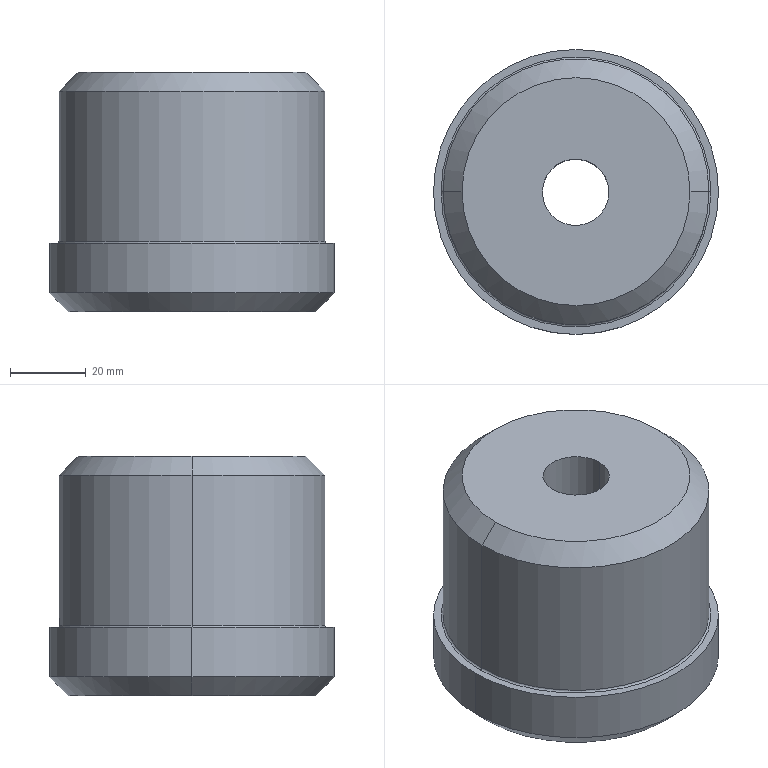Part | SolidWorks | features 3DProfileFeature 1, Chamfer 1, Extrusion 1, Fillet 1, HoleWzd 1, ICE 1 | 1 solid | 15 faces | box 75 x 75 x 63 mm | volume 232128 mm3 | cylinder 6 | cone 4 | plane 3 | torus 2 | commonest cylinder face diameters 17.5 x2 70 x2 75 x2
STEP:
#1=CARTESIAN_POINT('',(35.5,0.,0.));
#2=VERTEX_POINT('',#1);
#3=CARTESIAN_POINT('',(-35.5,0.,0.));
#4=VERTEX_POINT('',#3);
#5=CARTESIAN_POINT('',(0.,0.,0.));
#6=DIRECTION('',(0.,0.,-1.));
#7=DIRECTION('',(-1.,0.,0.));
#8=AXIS2_PLACEMENT_3D('',#5,#6,#7);
#9=CIRCLE('',#8,35.5);
#10=EDGE_CURVE('',#2,#4,#9,.T.);
#11=ORIENTED_EDGE('',*,*,#10,.F.);
#12=CARTESIAN_POINT('',(35.,0.,0.5));
#13=VERTEX_POINT('',#12);
#14=CARTESIAN_POINT('',(35.5,0.,0.5));
#15=DIRECTION('',(0.,1.,0.));
#16=DIRECTION('',(-1.,0.,0.));
#17=AXIS2_PLACEMENT_3D('',#14,#15,#16);
#18=CIRCLE('',#17,0.5);
#19=EDGE_CURVE('',#2,#13,#18,.T.);
#20=ORIENTED_EDGE('',*,*,#19,.T.);
#21=CARTESIAN_POINT('',(-35.,0.,0.5));
#22=VERTEX_POINT('',#21);
#23=CARTESIAN_POINT('',(0.,0.,0.5));
#24=DIRECTION('',(0.,0.,1.));
#25=DIRECTION('',(-1.,0.,0.));
#26=AXIS2_PLACEMENT_3D('',#23,#24,#25);
#27=CIRCLE('',#26,35.);
#28=EDGE_CURVE('',#22,#13,#27,.T.);
#29=ORIENTED_EDGE('',*,*,#28,.F.);
#30=CARTESIAN_POINT('',(-35.5,0.,0.5));
#31=DIRECTION('',(0.,-1.,0.));
#32=DIRECTION('',(0.,0.,-1.));
#33=AXIS2_PLACEMENT_3D('',#30,#31,#32);
#34=CIRCLE('',#33,0.5);
#35=EDGE_CURVE('',#4,#22,#34,.T.);
#36=ORIENTED_EDGE('',*,*,#35,.F.);
#37=EDGE_LOOP('',(#11,#20,#29,#36));
#38=FACE_OUTER_BOUND('',#37,.T.);
#39=CARTESIAN_POINT('',(0.,0.,0.5));
#40=DIRECTION('',(0.,0.,-1.));
#41=DIRECTION('',(-1.,0.,0.));
#42=AXIS2_PLACEMENT_3D('',#39,#40,#41);
#43=TOROIDAL_SURFACE('',#42,35.5,0.5);
#44=ADVANCED_FACE('',(#38),#43,.F.);
#45=CARTESIAN_POINT('',(-8.843,-0.1401,-18.));
#46=VERTEX_POINT('',#45);
#47=CARTESIAN_POINT('',(8.657,-0.1401,-18.));
#48=VERTEX_POINT('',#47);
#49=CARTESIAN_POINT('',(-0.09343,-0.1401,-18.));
#50=DIRECTION('',(0.,0.,1.));
#51=DIRECTION('',(1.,0.,0.));
#52=AXIS2_PLACEMENT_3D('',#49,#50,#51);
#53=CIRCLE('',#52,8.75);
#54=EDGE_CURVE('',#46,#48,#53,.T.);
#55=ORIENTED_EDGE('',*,*,#54,.F.);
#56=CARTESIAN_POINT('',(-8.843,-0.1401,45.));
#57=VERTEX_POINT('',#56);
#58=CARTESIAN_POINT('',(-8.843,-0.1401,45.));
#59=DIRECTION('',(0.,0.,1.));
#60=VECTOR('',#59,1000.);
#61=LINE('',#58,#60);
#62=EDGE_CURVE('',#46,#57,#61,.T.);
#63=ORIENTED_EDGE('',*,*,#62,.T.);
#64=CARTESIAN_POINT('',(8.657,-0.1401,45.));
#65=VERTEX_POINT('',#64);
#66=CARTESIAN_POINT('',(-0.09343,-0.1401,45.));
#67=DIRECTION('',(0.,0.,1.));
#68=DIRECTION('',(1.,0.,0.));
#69=AXIS2_PLACEMENT_3D('',#66,#67,#68);
#70=CIRCLE('',#69,8.75);
#71=EDGE_CURVE('',#57,#65,#70,.T.);
#72=ORIENTED_EDGE('',*,*,#71,.T.);
#73=CARTESIAN_POINT('',(8.657,-0.1401,45.));
#74=DIRECTION('',(0.,0.,1.));
#75=VECTOR('',#74,1000.);
#76=LINE('',#73,#75);
#77=EDGE_CURVE('',#48,#65,#76,.T.);
#78=ORIENTED_EDGE('',*,*,#77,.F.);
#79=EDGE_LOOP('',(#55,#63,#72,#78));
#80=FACE_OUTER_BOUND('',#79,.T.);
#81=CARTESIAN_POINT('',(-0.09343,-0.1401,45.));
#82=DIRECTION('',(0.,0.,1.));
#83=DIRECTION('',(1.,0.,0.));
#84=AXIS2_PLACEMENT_3D('',#81,#82,#83);
#85=CYLINDRICAL_SURFACE('',#84,8.75);
#86=ADVANCED_FACE('',(#80),#85,.F.);
#87=CARTESIAN_POINT('',(-32.5,0.,-18.));
#88=VERTEX_POINT('',#87);
#89=CARTESIAN_POINT('',(32.5,0.,-18.));
#90=VERTEX_POINT('',#89);
#91=CARTESIAN_POINT('',(0.,0.,-18.));
#92=DIRECTION('',(0.,0.,-1.));
#93=DIRECTION('',(-1.,0.,0.));
#94=AXIS2_PLACEMENT_3D('',#91,#92,#93);
#95=CIRCLE('',#94,32.5);
#96=EDGE_CURVE('',#88,#90,#95,.T.);
#97=ORIENTED_EDGE('',*,*,#96,.F.);
#98=CARTESIAN_POINT('',(-37.5,0.,-13.));
#99=VERTEX_POINT('',#98);
#100=CARTESIAN_POINT('',(-32.5,0.,-18.));
#101=DIRECTION('',(-0.7071,0.,0.7071));
#102=VECTOR('',#101,1000.);
#103=LINE('',#100,#102);
#104=EDGE_CURVE('',#88,#99,#103,.T.);
#105=ORIENTED_EDGE('',*,*,#104,.T.);
#106=CARTESIAN_POINT('',(37.5,0.,-13.));
#107=VERTEX_POINT('',#106);
#108=CARTESIAN_POINT('',(0.,0.,-13.));
#109=DIRECTION('',(0.,0.,1.));
#110=DIRECTION('',(-1.,0.,0.));
#111=AXIS2_PLACEMENT_3D('',#108,#109,#110);
#112=CIRCLE('',#111,37.5);
#113=EDGE_CURVE('',#107,#99,#112,.T.);
#114=ORIENTED_EDGE('',*,*,#113,.F.);
#115=CARTESIAN_POINT('',(32.5,0.,-18.));
#116=DIRECTION('',(0.7071,0.,0.7071));
#117=VECTOR('',#116,1000.);
#118=LINE('',#115,#117);
#119=EDGE_CURVE('',#90,#107,#118,.T.);
#120=ORIENTED_EDGE('',*,*,#119,.F.);
#121=EDGE_LOOP('',(#97,#105,#114,#120));
#122=FACE_OUTER_BOUND('',#121,.T.);
#123=CARTESIAN_POINT('',(0.,0.,-18.));
#124=DIRECTION('',(0.,0.,1.));
#125=DIRECTION('',(1.,0.,0.));
#126=AXIS2_PLACEMENT_3D('',#123,#124,#125);
#127=CONICAL_SURFACE('',#126,32.5,0.7854);
#128=ADVANCED_FACE('',(#122),#127,.T.);
#129=CARTESIAN_POINT('',(30.,0.,45.));
#130=VERTEX_POINT('',#129);
#131=CARTESIAN_POINT('',(-30.,0.,45.));
#132=VERTEX_POINT('',#131);
#133=CARTESIAN_POINT('',(0.,0.,45.));
#134=DIRECTION('',(0.,0.,1.));
#135=DIRECTION('',(1.,0.,0.));
#136=AXIS2_PLACEMENT_3D('',#133,#134,#135);
#137=CIRCLE('',#136,30.);
#138=EDGE_CURVE('',#130,#132,#137,.T.);
#139=ORIENTED_EDGE('',*,*,#138,.F.);
#140=CARTESIAN_POINT('',(35.,0.,40.));
#141=VERTEX_POINT('',#140);
#142=CARTESIAN_POINT('',(30.,0.,45.));
#143=DIRECTION('',(0.7071,0.,-0.7071));
#144=VECTOR('',#143,1000.);
#145=LINE('',#142,#144);
#146=EDGE_CURVE('',#130,#141,#145,.T.);
#147=ORIENTED_EDGE('',*,*,#146,.T.);
#148=CARTESIAN_POINT('',(-35.,0.,40.));
#149=VERTEX_POINT('',#148);
#150=CARTESIAN_POINT('',(0.,0.,40.));
#151=DIRECTION('',(0.,0.,-1.));
#152=DIRECTION('',(1.,0.,0.));
#153=AXIS2_PLACEMENT_3D('',#150,#151,#152);
#154=CIRCLE('',#153,35.);
#155=EDGE_CURVE('',#149,#141,#154,.T.);
#156=ORIENTED_EDGE('',*,*,#155,.F.);
#157=CARTESIAN_POINT('',(-30.,0.,45.));
#158=DIRECTION('',(-0.7071,0.,-0.7071));
#159=VECTOR('',#158,1000.);
#160=LINE('',#157,#159);
#161=EDGE_CURVE('',#132,#149,#160,.T.);
#162=ORIENTED_EDGE('',*,*,#161,.F.);
#163=EDGE_LOOP('',(#139,#147,#156,#162));
#164=FACE_OUTER_BOUND('',#163,.T.);
#165=CARTESIAN_POINT('',(0.,0.,45.));
#166=DIRECTION('',(0.,0.,-1.));
#167=DIRECTION('',(-1.,0.,0.));
#168=AXIS2_PLACEMENT_3D('',#165,#166,#167);
#169=CONICAL_SURFACE('',#168,30.,0.7854);
#170=ADVANCED_FACE('',(#164),#169,.T.);
#171=ORIENTED_EDGE('',*,*,#113,.T.);
#172=CARTESIAN_POINT('',(-37.5,0.,0.));
#173=VERTEX_POINT('',#172);
#174=CARTESIAN_POINT('',(-37.5,0.,-18.));
#175=DIRECTION('',(0.,0.,1.));
#176=VECTOR('',#175,1000.);
#177=LINE('',#174,#176);
#178=EDGE_CURVE('',#99,#173,#177,.T.);
#179=ORIENTED_EDGE('',*,*,#178,.T.);
#180=CARTESIAN_POINT('',(37.5,0.,0.));
#181=VERTEX_POINT('',#180);
#182=CARTESIAN_POINT('',(0.,0.,0.));
#183=DIRECTION('',(0.,0.,-1.));
#184=DIRECTION('',(-1.,0.,0.));
#185=AXIS2_PLACEMENT_3D('',#182,#183,#184);
#186=CIRCLE('',#185,37.5);
#187=EDGE_CURVE('',#173,#181,#186,.T.);
#188=ORIENTED_EDGE('',*,*,#187,.T.);
#189=CARTESIAN_POINT('',(37.5,0.,-18.));
#190=DIRECTION('',(0.,0.,1.));
#191=VECTOR('',#190,1000.);
#192=LINE('',#189,#191);
#193=EDGE_CURVE('',#107,#181,#192,.T.);
#194=ORIENTED_EDGE('',*,*,#193,.F.);
#195=EDGE_LOOP('',(#171,#179,#188,#194));
#196=FACE_OUTER_BOUND('',#195,.T.);
#197=CARTESIAN_POINT('',(0.,0.,-18.));
#198=DIRECTION('',(0.,0.,1.));
#199=DIRECTION('',(1.,0.,0.));
#200=AXIS2_PLACEMENT_3D('',#197,#198,#199);
#201=CYLINDRICAL_SURFACE('',#200,37.5);
#202=ADVANCED_FACE('',(#196),#201,.T.);
#203=ORIENTED_EDGE('',*,*,#155,.T.);
#204=CARTESIAN_POINT('',(35.,0.,45.));
#205=DIRECTION('',(0.,0.,-1.));
#206=VECTOR('',#205,1000.);
#207=LINE('',#204,#206);
#208=EDGE_CURVE('',#141,#13,#207,.T.);
#209=ORIENTED_EDGE('',*,*,#208,.T.);
#210=CARTESIAN_POINT('',(0.,0.,0.5));
#211=DIRECTION('',(0.,0.,1.));
#212=DIRECTION('',(-1.,0.,0.));
#213=AXIS2_PLACEMENT_3D('',#210,#211,#212);
#214=CIRCLE('',#213,35.);
#215=EDGE_CURVE('',#13,#22,#214,.T.);
#216=ORIENTED_EDGE('',*,*,#215,.T.);
#217=CARTESIAN_POINT('',(-35.,0.,45.));
#218=DIRECTION('',(0.,0.,-1.));
#219=VECTOR('',#218,1000.);
#220=LINE('',#217,#219);
#221=EDGE_CURVE('',#149,#22,#220,.T.);
#222=ORIENTED_EDGE('',*,*,#221,.F.);
#223=EDGE_LOOP('',(#203,#209,#216,#222));
#224=FACE_OUTER_BOUND('',#223,.T.);
#225=CARTESIAN_POINT('',(0.,0.,45.));
#226=DIRECTION('',(0.,0.,-1.));
#227=DIRECTION('',(-1.,0.,0.));
#228=AXIS2_PLACEMENT_3D('',#225,#226,#227);
#229=CYLINDRICAL_SURFACE('',#228,35.);
#230=ADVANCED_FACE('',(#224),#229,.T.);
#231=ORIENTED_EDGE('',*,*,#208,.F.);
#232=CARTESIAN_POINT('',(0.,0.,40.));
#233=DIRECTION('',(0.,0.,-1.));
#234=DIRECTION('',(1.,0.,0.));
#235=AXIS2_PLACEMENT_3D('',#232,#233,#234);
#236=CIRCLE('',#235,35.);
#237=EDGE_CURVE('',#141,#149,#236,.T.);
#238=ORIENTED_EDGE('',*,*,#237,.T.);
#239=ORIENTED_EDGE('',*,*,#221,.T.);
#240=ORIENTED_EDGE('',*,*,#28,.T.);
#241=EDGE_LOOP('',(#231,#238,#239,#240));
#242=FACE_OUTER_BOUND('',#241,.T.);
#243=CARTESIAN_POINT('',(0.,0.,45.));
#244=DIRECTION('',(0.,0.,-1.));
#245=DIRECTION('',(-1.,0.,0.));
#246=AXIS2_PLACEMENT_3D('',#243,#244,#245);
#247=CYLINDRICAL_SURFACE('',#246,35.);
#248=ADVANCED_FACE('',(#242),#247,.T.);
#249=CARTESIAN_POINT('',(-0.09343,-0.1401,45.));
#250=DIRECTION('',(0.,0.,1.));
#251=DIRECTION('',(1.,0.,0.));
#252=AXIS2_PLACEMENT_3D('',#249,#250,#251);
#253=CIRCLE('',#252,8.75);
#254=EDGE_CURVE('',#65,#57,#253,.T.);
#255=ORIENTED_EDGE('',*,*,#254,.F.);
#256=ORIENTED_EDGE('',*,*,#71,.F.);
#257=EDGE_LOOP('',(#255,#256));
#258=FACE_BOUND('',#257,.T.);
#259=CARTESIAN_POINT('',(0.,0.,45.));
#260=DIRECTION('',(0.,0.,1.));
#261=DIRECTION('',(1.,0.,0.));
#262=AXIS2_PLACEMENT_3D('',#259,#260,#261);
#263=CIRCLE('',#262,30.);
#264=EDGE_CURVE('',#132,#130,#263,.T.);
#265=ORIENTED_EDGE('',*,*,#264,.T.);
#266=ORIENTED_EDGE('',*,*,#138,.T.);
#267=EDGE_LOOP('',(#265,#266));
#268=FACE_OUTER_BOUND('',#267,.T.);
#269=CARTESIAN_POINT('',(0.,0.,45.));
#270=DIRECTION('',(0.,0.,1.));
#271=DIRECTION('',(1.,0.,0.));
#272=AXIS2_PLACEMENT_3D('',#269,#270,#271);
#273=PLANE('',#272);
#274=ADVANCED_FACE('',(#258,#268),#273,.T.);
#275=ORIENTED_EDGE('',*,*,#178,.F.);
#276=CARTESIAN_POINT('',(0.,0.,-13.));
#277=DIRECTION('',(0.,0.,1.));
#278=DIRECTION('',(-1.,0.,0.));
#279=AXIS2_PLACEMENT_3D('',#276,#277,#278);
#280=CIRCLE('',#279,37.5);
#281=EDGE_CURVE('',#99,#107,#280,.T.);
#282=ORIENTED_EDGE('',*,*,#281,.T.);
#283=ORIENTED_EDGE('',*,*,#193,.T.);
#284=CARTESIAN_POINT('',(0.,0.,0.));
#285=DIRECTION('',(0.,0.,-1.));
#286=DIRECTION('',(-1.,0.,0.));
#287=AXIS2_PLACEMENT_3D('',#284,#285,#286);
#288=CIRCLE('',#287,37.5);
#289=EDGE_CURVE('',#181,#173,#288,.T.);
#290=ORIENTED_EDGE('',*,*,#289,.T.);
#291=EDGE_LOOP('',(#275,#282,#283,#290));
#292=FACE_OUTER_BOUND('',#291,.T.);
#293=CARTESIAN_POINT('',(0.,0.,-18.));
#294=DIRECTION('',(0.,0.,1.));
#295=DIRECTION('',(1.,0.,0.));
#296=AXIS2_PLACEMENT_3D('',#293,#294,#295);
#297=CYLINDRICAL_SURFACE('',#296,37.5);
#298=ADVANCED_FACE('',(#292),#297,.T.);
#299=CARTESIAN_POINT('',(-0.09343,-0.1401,-18.));
#300=DIRECTION('',(0.,0.,1.));
#301=DIRECTION('',(1.,0.,0.));
#302=AXIS2_PLACEMENT_3D('',#299,#300,#301);
#303=CIRCLE('',#302,8.75);
#304=EDGE_CURVE('',#48,#46,#303,.T.);
#305=ORIENTED_EDGE('',*,*,#304,.T.);
#306=ORIENTED_EDGE('',*,*,#54,.T.);
#307=EDGE_LOOP('',(#305,#306));
#308=FACE_BOUND('',#307,.T.);
#309=CARTESIAN_POINT('',(0.,0.,-18.));
#310=DIRECTION('',(0.,0.,-1.));
#311=DIRECTION('',(-1.,0.,0.));
#312=AXIS2_PLACEMENT_3D('',#309,#310,#311);
#313=CIRCLE('',#312,32.5);
#314=EDGE_CURVE('',#90,#88,#313,.T.);
#315=ORIENTED_EDGE('',*,*,#314,.T.);
#316=ORIENTED_EDGE('',*,*,#96,.T.);
#317=EDGE_LOOP('',(#315,#316));
#318=FACE_OUTER_BOUND('',#317,.T.);
#319=CARTESIAN_POINT('',(0.,0.,-18.));
#320=DIRECTION('',(0.,0.,-1.));
#321=DIRECTION('',(-1.,0.,0.));
#322=AXIS2_PLACEMENT_3D('',#319,#320,#321);
#323=PLANE('',#322);
#324=ADVANCED_FACE('',(#308,#318),#323,.T.);
#325=CARTESIAN_POINT('',(0.,0.,0.));
#326=DIRECTION('',(0.,0.,-1.));
#327=DIRECTION('',(-1.,0.,0.));
#328=AXIS2_PLACEMENT_3D('',#325,#326,#327);
#329=CIRCLE('',#328,35.5);
#330=EDGE_CURVE('',#4,#2,#329,.T.);
#331=ORIENTED_EDGE('',*,*,#330,.T.);
#332=ORIENTED_EDGE('',*,*,#10,.T.);
#333=EDGE_LOOP('',(#331,#332));
#334=FACE_BOUND('',#333,.T.);
#335=ORIENTED_EDGE('',*,*,#289,.F.);
#336=ORIENTED_EDGE('',*,*,#187,.F.);
#337=EDGE_LOOP('',(#335,#336));
#338=FACE_OUTER_BOUND('',#337,.T.);
#339=CARTESIAN_POINT('',(0.,0.,0.));
#340=DIRECTION('',(0.,0.,-1.));
#341=DIRECTION('',(-1.,0.,0.));
#342=AXIS2_PLACEMENT_3D('',#339,#340,#341);
#343=PLANE('',#342);
#344=ADVANCED_FACE('',(#334,#338),#343,.F.);
#345=ORIENTED_EDGE('',*,*,#146,.F.);
#346=ORIENTED_EDGE('',*,*,#264,.F.);
#347=ORIENTED_EDGE('',*,*,#161,.T.);
#348=ORIENTED_EDGE('',*,*,#237,.F.);
#349=EDGE_LOOP('',(#345,#346,#347,#348));
#350=FACE_OUTER_BOUND('',#349,.T.);
#351=CARTESIAN_POINT('',(0.,0.,45.));
#352=DIRECTION('',(0.,0.,-1.));
#353=DIRECTION('',(-1.,0.,0.));
#354=AXIS2_PLACEMENT_3D('',#351,#352,#353);
#355=CONICAL_SURFACE('',#354,30.,0.7854);
#356=ADVANCED_FACE('',(#350),#355,.T.);
#357=ORIENTED_EDGE('',*,*,#104,.F.);
#358=ORIENTED_EDGE('',*,*,#314,.F.);
#359=ORIENTED_EDGE('',*,*,#119,.T.);
#360=ORIENTED_EDGE('',*,*,#281,.F.);
#361=EDGE_LOOP('',(#357,#358,#359,#360));
#362=FACE_OUTER_BOUND('',#361,.T.);
#363=CARTESIAN_POINT('',(0.,0.,-18.));
#364=DIRECTION('',(0.,0.,1.));
#365=DIRECTION('',(1.,0.,0.));
#366=AXIS2_PLACEMENT_3D('',#363,#364,#365);
#367=CONICAL_SURFACE('',#366,32.5,0.7854);
#368=ADVANCED_FACE('',(#362),#367,.T.);
#369=ORIENTED_EDGE('',*,*,#62,.F.);
#370=ORIENTED_EDGE('',*,*,#304,.F.);
#371=ORIENTED_EDGE('',*,*,#77,.T.);
#372=ORIENTED_EDGE('',*,*,#254,.T.);
#373=EDGE_LOOP('',(#369,#370,#371,#372));
#374=FACE_OUTER_BOUND('',#373,.T.);
#375=CARTESIAN_POINT('',(-0.09343,-0.1401,45.));
#376=DIRECTION('',(0.,0.,1.));
#377=DIRECTION('',(1.,0.,0.));
#378=AXIS2_PLACEMENT_3D('',#375,#376,#377);
#379=CYLINDRICAL_SURFACE('',#378,8.75);
#380=ADVANCED_FACE('',(#374),#379,.F.);
#381=ORIENTED_EDGE('',*,*,#19,.F.);
#382=ORIENTED_EDGE('',*,*,#330,.F.);
#383=ORIENTED_EDGE('',*,*,#35,.T.);
#384=ORIENTED_EDGE('',*,*,#215,.F.);
#385=EDGE_LOOP('',(#381,#382,#383,#384));
#386=FACE_OUTER_BOUND('',#385,.T.);
#387=CARTESIAN_POINT('',(0.,0.,0.5));
#388=DIRECTION('',(0.,0.,-1.));
#389=DIRECTION('',(-1.,0.,0.));
#390=AXIS2_PLACEMENT_3D('',#387,#388,#389);
#391=TOROIDAL_SURFACE('',#390,35.5,0.5);
#392=ADVANCED_FACE('',(#386),#391,.F.);
#393=CLOSED_SHELL('',(#44,#86,#128,#170,#202,#230,#248,#274,#298,#324,#344,#356,#368,#380,#392));
#394=MANIFOLD_SOLID_BREP('',#393);
#395=CARTESIAN_POINT('',(0.,0.,0.));
#396=DIRECTION('',(0.,0.,1.));
#397=DIRECTION('',(1.,0.,0.));
#398=AXIS2_PLACEMENT_3D('',#395,#396,#397);
#399=(LENGTH_UNIT()NAMED_UNIT(*)SI_UNIT(.MILLI.,.METRE.));
#400=UNCERTAINTY_MEASURE_WITH_UNIT(LENGTH_MEASURE(0.00001),#399,'','');
#401=(NAMED_UNIT(*)PLANE_ANGLE_UNIT()SI_UNIT($,.RADIAN.));
#402=(NAMED_UNIT(*)SI_UNIT($,.STERADIAN.)SOLID_ANGLE_UNIT());
#403=(GEOMETRIC_REPRESENTATION_CONTEXT(3)GLOBAL_UNCERTAINTY_ASSIGNED_CONTEXT((#400))GLOBAL_UNIT_ASSIGNED_CONTEXT((#399,#401,#402))REPRESENTATION_CONTEXT('',''));
#404=ADVANCED_BREP_SHAPE_REPRESENTATION('',(#394,#398),#403);